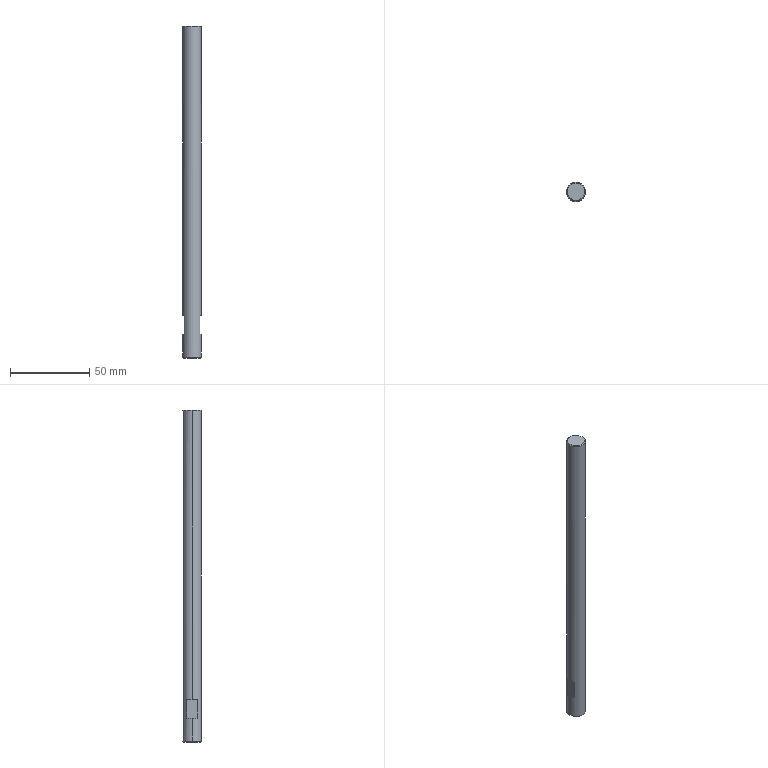Part | STEP file | 2010 Bag feed support shaft | 1 solid | 18 faces | box 12 x 12 x 210 mm | volume 23133 mm3 | plane 8 | cone 6 | cylinder 4 | commonest cylinder face diameters 5 x2 12 x2
STEP:
#1=CARTESIAN_POINT('',(0.,0.,0.));
#2=DIRECTION('',(0.,0.,1.));
#3=DIRECTION('',(1.,0.,0.));
#4=AXIS2_PLACEMENT_3D('',#1,#2,#3);
#5=CARTESIAN_POINT('',(5.5,0.,210.));
#6=VERTEX_POINT('',#5);
#7=CARTESIAN_POINT('',(-5.5,0.,210.));
#8=VERTEX_POINT('',#7);
#9=CARTESIAN_POINT('',(0.,0.,210.));
#10=DIRECTION('',(0.,0.,1.));
#11=DIRECTION('',(1.,0.,0.));
#12=AXIS2_PLACEMENT_3D('',#9,#10,#11);
#13=CIRCLE('',#12,5.5);
#14=CARTESIAN_POINT('',(0.,0.,210.));
#15=DIRECTION('',(0.,0.,-1.));
#16=DIRECTION('',(-1.,0.,0.));
#17=AXIS2_PLACEMENT_3D('',#14,#15,#16);
#18=CONICAL_SURFACE('',#17,5.5,0.7854);
#19=CARTESIAN_POINT('',(3.142,0.));
#20=DIRECTION('',(-1.,0.));
#21=VECTOR('',#20,1.);
#22=LINE('',#19,#21);
#23=(GEOMETRIC_REPRESENTATION_CONTEXT(2)PARAMETRIC_REPRESENTATION_CONTEXT()REPRESENTATION_CONTEXT('',''));
#24=DEFINITIONAL_REPRESENTATION('',(#22),#23);
#25=PCURVE('',#18,#24);
#26=CARTESIAN_POINT('',(0.,0.,210.));
#27=DIRECTION('',(0.,0.,1.));
#28=DIRECTION('',(1.,0.,0.));
#29=AXIS2_PLACEMENT_3D('',#26,#27,#28);
#30=PLANE('',#29);
#31=CARTESIAN_POINT('',(0.,0.));
#32=DIRECTION('',(1.,0.));
#33=AXIS2_PLACEMENT_2D('',#31,#32);
#34=CIRCLE('',#33,5.5);
#35=(GEOMETRIC_REPRESENTATION_CONTEXT(2)PARAMETRIC_REPRESENTATION_CONTEXT()REPRESENTATION_CONTEXT('',''));
#36=DEFINITIONAL_REPRESENTATION('',(#34),#35);
#37=PCURVE('',#30,#36);
#38=SURFACE_CURVE('',#13,(#25,#37),.PCURVE_S1.);
#39=EDGE_CURVE('',#6,#8,#38,.T.);
#40=ORIENTED_EDGE('',*,*,#39,.F.);
#41=CARTESIAN_POINT('',(6.,0.,209.5));
#42=VERTEX_POINT('',#41);
#43=CARTESIAN_POINT('',(5.5,0.,210.));
#44=DIRECTION('',(0.7071,0.,-0.7071));
#45=VECTOR('',#44,1.);
#46=LINE('',#43,#45);
#47=CARTESIAN_POINT('',(3.142,0.));
#48=DIRECTION('',(0.,1.));
#49=VECTOR('',#48,1.);
#50=LINE('',#47,#49);
#51=(GEOMETRIC_REPRESENTATION_CONTEXT(2)PARAMETRIC_REPRESENTATION_CONTEXT()REPRESENTATION_CONTEXT('',''));
#52=DEFINITIONAL_REPRESENTATION('',(#50),#51);
#53=PCURVE('',#18,#52);
#54=CARTESIAN_POINT('',(0.,0.,210.));
#55=DIRECTION('',(0.,0.,-1.));
#56=DIRECTION('',(-1.,0.,0.));
#57=AXIS2_PLACEMENT_3D('',#54,#55,#56);
#58=CONICAL_SURFACE('',#57,5.5,0.7854);
#59=CARTESIAN_POINT('',(3.142,0.));
#60=DIRECTION('',(0.,1.));
#61=VECTOR('',#60,1.);
#62=LINE('',#59,#61);
#63=(GEOMETRIC_REPRESENTATION_CONTEXT(2)PARAMETRIC_REPRESENTATION_CONTEXT()REPRESENTATION_CONTEXT('',''));
#64=DEFINITIONAL_REPRESENTATION('',(#62),#63);
#65=PCURVE('',#58,#64);
#66=SURFACE_CURVE('',#46,(#53,#65),.PCURVE_S1.);
#67=EDGE_CURVE('',#6,#42,#66,.T.);
#68=ORIENTED_EDGE('',*,*,#67,.T.);
#69=CARTESIAN_POINT('',(-6.,0.,209.5));
#70=VERTEX_POINT('',#69);
#71=CARTESIAN_POINT('',(0.,0.,209.5));
#72=DIRECTION('',(0.,0.,-1.));
#73=DIRECTION('',(1.,0.,0.));
#74=AXIS2_PLACEMENT_3D('',#71,#72,#73);
#75=CIRCLE('',#74,6.);
#76=CARTESIAN_POINT('',(-3.142,0.5));
#77=DIRECTION('',(1.,0.));
#78=VECTOR('',#77,1.);
#79=LINE('',#76,#78);
#80=(GEOMETRIC_REPRESENTATION_CONTEXT(2)PARAMETRIC_REPRESENTATION_CONTEXT()REPRESENTATION_CONTEXT('',''));
#81=DEFINITIONAL_REPRESENTATION('',(#79),#80);
#82=PCURVE('',#18,#81);
#83=CARTESIAN_POINT('',(0.,0.,210.));
#84=DIRECTION('',(0.,0.,-1.));
#85=DIRECTION('',(-1.,0.,0.));
#86=AXIS2_PLACEMENT_3D('',#83,#84,#85);
#87=CYLINDRICAL_SURFACE('',#86,6.);
#88=CARTESIAN_POINT('',(-3.142,0.5));
#89=DIRECTION('',(1.,0.));
#90=VECTOR('',#89,1.);
#91=LINE('',#88,#90);
#92=(GEOMETRIC_REPRESENTATION_CONTEXT(2)PARAMETRIC_REPRESENTATION_CONTEXT()REPRESENTATION_CONTEXT('',''));
#93=DEFINITIONAL_REPRESENTATION('',(#91),#92);
#94=PCURVE('',#87,#93);
#95=SURFACE_CURVE('',#75,(#82,#94),.PCURVE_S1.);
#96=EDGE_CURVE('',#70,#42,#95,.T.);
#97=ORIENTED_EDGE('',*,*,#96,.F.);
#98=CARTESIAN_POINT('',(-5.5,0.,210.));
#99=DIRECTION('',(-0.7071,0.,-0.7071));
#100=VECTOR('',#99,1.);
#101=LINE('',#98,#100);
#102=CARTESIAN_POINT('',(0.,0.));
#103=DIRECTION('',(0.,1.));
#104=VECTOR('',#103,1.);
#105=LINE('',#102,#104);
#106=(GEOMETRIC_REPRESENTATION_CONTEXT(2)PARAMETRIC_REPRESENTATION_CONTEXT()REPRESENTATION_CONTEXT('',''));
#107=DEFINITIONAL_REPRESENTATION('',(#105),#106);
#108=PCURVE('',#18,#107);
#109=CARTESIAN_POINT('',(6.283,0.));
#110=DIRECTION('',(0.,1.));
#111=VECTOR('',#110,1.);
#112=LINE('',#109,#111);
#113=(GEOMETRIC_REPRESENTATION_CONTEXT(2)PARAMETRIC_REPRESENTATION_CONTEXT()REPRESENTATION_CONTEXT('',''));
#114=DEFINITIONAL_REPRESENTATION('',(#112),#113);
#115=PCURVE('',#58,#114);
#116=SURFACE_CURVE('',#101,(#108,#115),.PCURVE_S1.);
#117=EDGE_CURVE('',#8,#70,#116,.T.);
#118=ORIENTED_EDGE('',*,*,#117,.F.);
#119=EDGE_LOOP('',(#40,#68,#97,#118));
#120=FACE_BOUND('',#119,.T.);
#121=ADVANCED_FACE('',(#120),#18,.T.);
#122=CARTESIAN_POINT('',(-5.5,0.,0.));
#123=VERTEX_POINT('',#122);
#124=CARTESIAN_POINT('',(5.5,0.,0.));
#125=VERTEX_POINT('',#124);
#126=CARTESIAN_POINT('',(0.,0.,0.));
#127=DIRECTION('',(0.,0.,-1.));
#128=DIRECTION('',(1.,0.,0.));
#129=AXIS2_PLACEMENT_3D('',#126,#127,#128);
#130=CIRCLE('',#129,5.5);
#131=CARTESIAN_POINT('',(0.,0.,0.5));
#132=DIRECTION('',(0.,0.,1.));
#133=DIRECTION('',(1.,0.,0.));
#134=AXIS2_PLACEMENT_3D('',#131,#132,#133);
#135=CONICAL_SURFACE('',#134,6.,0.7854);
#136=CARTESIAN_POINT('',(6.283,-0.5));
#137=DIRECTION('',(-1.,0.));
#138=VECTOR('',#137,1.);
#139=LINE('',#136,#138);
#140=(GEOMETRIC_REPRESENTATION_CONTEXT(2)PARAMETRIC_REPRESENTATION_CONTEXT()REPRESENTATION_CONTEXT('',''));
#141=DEFINITIONAL_REPRESENTATION('',(#139),#140);
#142=PCURVE('',#135,#141);
#143=CARTESIAN_POINT('',(0.,0.,0.));
#144=DIRECTION('',(0.,0.,1.));
#145=DIRECTION('',(1.,0.,0.));
#146=AXIS2_PLACEMENT_3D('',#143,#144,#145);
#147=PLANE('',#146);
#148=CARTESIAN_POINT('',(5.5,0.));
#149=CARTESIAN_POINT('',(5.5,-9.526));
#150=CARTESIAN_POINT('',(-2.75,-4.763));
#151=CARTESIAN_POINT('',(-11.,0.));
#152=CARTESIAN_POINT('',(-2.75,4.763));
#153=CARTESIAN_POINT('',(5.5,9.526));
#154=CARTESIAN_POINT('',(5.5,0.));
#155=(BOUNDED_CURVE()B_SPLINE_CURVE(2,(#148,#149,#150,#151,#152,#153,#154),.UNSPECIFIED.,.T.,.F.)B_SPLINE_CURVE_WITH_KNOTS((1,2,2,2,2,1),(-2.094,0.,2.094,4.189,6.283,8.378),.UNSPECIFIED.)CURVE()GEOMETRIC_REPRESENTATION_ITEM()RATIONAL_B_SPLINE_CURVE((1.,0.5,1.,0.5,1.,0.5,1.))REPRESENTATION_ITEM(''));
#156=(GEOMETRIC_REPRESENTATION_CONTEXT(2)PARAMETRIC_REPRESENTATION_CONTEXT()REPRESENTATION_CONTEXT('',''));
#157=DEFINITIONAL_REPRESENTATION('',(#155),#156);
#158=PCURVE('',#147,#157);
#159=SURFACE_CURVE('',#130,(#142,#158),.PCURVE_S1.);
#160=EDGE_CURVE('',#123,#125,#159,.T.);
#161=ORIENTED_EDGE('',*,*,#160,.F.);
#162=CARTESIAN_POINT('',(-6.,0.,0.5));
#163=VERTEX_POINT('',#162);
#164=CARTESIAN_POINT('',(-6.,0.,0.5));
#165=DIRECTION('',(-0.7071,0.,0.7071));
#166=VECTOR('',#165,1.);
#167=LINE('',#164,#166);
#168=CARTESIAN_POINT('',(3.142,0.));
#169=DIRECTION('',(0.,1.));
#170=VECTOR('',#169,1.);
#171=LINE('',#168,#170);
#172=(GEOMETRIC_REPRESENTATION_CONTEXT(2)PARAMETRIC_REPRESENTATION_CONTEXT()REPRESENTATION_CONTEXT('',''));
#173=DEFINITIONAL_REPRESENTATION('',(#171),#172);
#174=PCURVE('',#135,#173);
#175=CARTESIAN_POINT('',(0.,0.,0.5));
#176=DIRECTION('',(0.,0.,1.));
#177=DIRECTION('',(1.,0.,0.));
#178=AXIS2_PLACEMENT_3D('',#175,#176,#177);
#179=CONICAL_SURFACE('',#178,6.,0.7854);
#180=CARTESIAN_POINT('',(3.142,0.));
#181=DIRECTION('',(0.,1.));
#182=VECTOR('',#181,1.);
#183=LINE('',#180,#182);
#184=(GEOMETRIC_REPRESENTATION_CONTEXT(2)PARAMETRIC_REPRESENTATION_CONTEXT()REPRESENTATION_CONTEXT('',''));
#185=DEFINITIONAL_REPRESENTATION('',(#183),#184);
#186=PCURVE('',#179,#185);
#187=SURFACE_CURVE('',#167,(#174,#186),.PCURVE_S1.);
#188=EDGE_CURVE('',#123,#163,#187,.T.);
#189=ORIENTED_EDGE('',*,*,#188,.T.);
#190=CARTESIAN_POINT('',(6.,0.,0.5));
#191=VERTEX_POINT('',#190);
#192=CARTESIAN_POINT('',(0.,0.,0.5));
#193=DIRECTION('',(0.,0.,1.));
#194=DIRECTION('',(1.,0.,0.));
#195=AXIS2_PLACEMENT_3D('',#192,#193,#194);
#196=CIRCLE('',#195,6.);
#197=CARTESIAN_POINT('',(0.,0.));
#198=DIRECTION('',(1.,0.));
#199=VECTOR('',#198,1.);
#200=LINE('',#197,#199);
#201=(GEOMETRIC_REPRESENTATION_CONTEXT(2)PARAMETRIC_REPRESENTATION_CONTEXT()REPRESENTATION_CONTEXT('',''));
#202=DEFINITIONAL_REPRESENTATION('',(#200),#201);
#203=PCURVE('',#135,#202);
#204=CARTESIAN_POINT('',(3.142,209.5));
#205=DIRECTION('',(-1.,0.));
#206=VECTOR('',#205,1.);
#207=LINE('',#204,#206);
#208=(GEOMETRIC_REPRESENTATION_CONTEXT(2)PARAMETRIC_REPRESENTATION_CONTEXT()REPRESENTATION_CONTEXT('',''));
#209=DEFINITIONAL_REPRESENTATION('',(#207),#208);
#210=PCURVE('',#87,#209);
#211=SURFACE_CURVE('',#196,(#203,#210),.PCURVE_S1.);
#212=EDGE_CURVE('',#191,#163,#211,.T.);
#213=ORIENTED_EDGE('',*,*,#212,.F.);
#214=CARTESIAN_POINT('',(6.,0.,0.5));
#215=DIRECTION('',(0.7071,0.,0.7071));
#216=VECTOR('',#215,1.);
#217=LINE('',#214,#216);
#218=CARTESIAN_POINT('',(0.,0.));
#219=DIRECTION('',(0.,1.));
#220=VECTOR('',#219,1.);
#221=LINE('',#218,#220);
#222=(GEOMETRIC_REPRESENTATION_CONTEXT(2)PARAMETRIC_REPRESENTATION_CONTEXT()REPRESENTATION_CONTEXT('',''));
#223=DEFINITIONAL_REPRESENTATION('',(#221),#222);
#224=PCURVE('',#135,#223);
#225=CARTESIAN_POINT('',(6.283,0.));
#226=DIRECTION('',(0.,1.));
#227=VECTOR('',#226,1.);
#228=LINE('',#225,#227);
#229=(GEOMETRIC_REPRESENTATION_CONTEXT(2)PARAMETRIC_REPRESENTATION_CONTEXT()REPRESENTATION_CONTEXT('',''));
#230=DEFINITIONAL_REPRESENTATION('',(#228),#229);
#231=PCURVE('',#179,#230);
#232=SURFACE_CURVE('',#217,(#224,#231),.PCURVE_S1.);
#233=EDGE_CURVE('',#125,#191,#232,.T.);
#234=ORIENTED_EDGE('',*,*,#233,.F.);
#235=EDGE_LOOP('',(#161,#189,#213,#234));
#236=FACE_BOUND('',#235,.T.);
#237=ADVANCED_FACE('',(#236),#135,.T.);
#238=CARTESIAN_POINT('',(-2.5,0.,25.));
#239=VERTEX_POINT('',#238);
#240=CARTESIAN_POINT('',(-2.5,0.,0.));
#241=VERTEX_POINT('',#240);
#242=CARTESIAN_POINT('',(-2.5,0.,0.));
#243=DIRECTION('',(0.,0.,-1.));
#244=VECTOR('',#243,1.);
#245=LINE('',#242,#244);
#246=CARTESIAN_POINT('',(0.,0.,0.));
#247=DIRECTION('',(0.,0.,-1.));
#248=DIRECTION('',(-1.,0.,0.));
#249=AXIS2_PLACEMENT_3D('',#246,#247,#248);
#250=CYLINDRICAL_SURFACE('',#249,2.5);
#251=CARTESIAN_POINT('',(6.283,0.));
#252=DIRECTION('',(0.,1.));
#253=VECTOR('',#252,1.);
#254=LINE('',#251,#253);
#255=(GEOMETRIC_REPRESENTATION_CONTEXT(2)PARAMETRIC_REPRESENTATION_CONTEXT()REPRESENTATION_CONTEXT('',''));
#256=DEFINITIONAL_REPRESENTATION('',(#254),#255);
#257=PCURVE('',#250,#256);
#258=CARTESIAN_POINT('',(0.,0.,0.));
#259=DIRECTION('',(0.,0.,-1.));
#260=DIRECTION('',(-1.,0.,0.));
#261=AXIS2_PLACEMENT_3D('',#258,#259,#260);
#262=CYLINDRICAL_SURFACE('',#261,2.5);
#263=CARTESIAN_POINT('',(0.,0.));
#264=DIRECTION('',(0.,1.));
#265=VECTOR('',#264,1.);
#266=LINE('',#263,#265);
#267=(GEOMETRIC_REPRESENTATION_CONTEXT(2)PARAMETRIC_REPRESENTATION_CONTEXT()REPRESENTATION_CONTEXT('',''));
#268=DEFINITIONAL_REPRESENTATION('',(#266),#267);
#269=PCURVE('',#262,#268);
#270=SURFACE_CURVE('',#245,(#257,#269),.PCURVE_S1.);
#271=EDGE_CURVE('',#239,#241,#270,.T.);
#272=ORIENTED_EDGE('',*,*,#271,.T.);
#273=CARTESIAN_POINT('',(2.5,0.,0.));
#274=VERTEX_POINT('',#273);
#275=CARTESIAN_POINT('',(0.,0.,0.));
#276=DIRECTION('',(0.,0.,-1.));
#277=DIRECTION('',(-1.,0.,0.));
#278=AXIS2_PLACEMENT_3D('',#275,#276,#277);
#279=CIRCLE('',#278,2.5);
#280=CARTESIAN_POINT('',(0.,0.));
#281=DIRECTION('',(1.,0.));
#282=VECTOR('',#281,1.);
#283=LINE('',#280,#282);
#284=(GEOMETRIC_REPRESENTATION_CONTEXT(2)PARAMETRIC_REPRESENTATION_CONTEXT()REPRESENTATION_CONTEXT('',''));
#285=DEFINITIONAL_REPRESENTATION('',(#283),#284);
#286=PCURVE('',#250,#285);
#287=CARTESIAN_POINT('',(-2.5,0.));
#288=CARTESIAN_POINT('',(-2.5,4.33));
#289=CARTESIAN_POINT('',(1.25,2.165));
#290=CARTESIAN_POINT('',(5.,0.));
#291=CARTESIAN_POINT('',(1.25,-2.165));
#292=CARTESIAN_POINT('',(-2.5,-4.33));
#293=CARTESIAN_POINT('',(-2.5,0.));
#294=(BOUNDED_CURVE()B_SPLINE_CURVE(2,(#287,#288,#289,#290,#291,#292,#293),.UNSPECIFIED.,.T.,.F.)B_SPLINE_CURVE_WITH_KNOTS((1,2,2,2,2,1),(-2.094,0.,2.094,4.189,6.283,8.378),.UNSPECIFIED.)CURVE()GEOMETRIC_REPRESENTATION_ITEM()RATIONAL_B_SPLINE_CURVE((1.,0.5,1.,0.5,1.,0.5,1.))REPRESENTATION_ITEM(''));
#295=(GEOMETRIC_REPRESENTATION_CONTEXT(2)PARAMETRIC_REPRESENTATION_CONTEXT()REPRESENTATION_CONTEXT('',''));
#296=DEFINITIONAL_REPRESENTATION('',(#294),#295);
#297=PCURVE('',#147,#296);
#298=SURFACE_CURVE('',#279,(#286,#297),.PCURVE_S1.);
#299=EDGE_CURVE('',#274,#241,#298,.T.);
#300=ORIENTED_EDGE('',*,*,#299,.F.);
#301=CARTESIAN_POINT('',(2.5,0.,25.));
#302=VERTEX_POINT('',#301);
#303=CARTESIAN_POINT('',(2.5,0.,0.));
#304=DIRECTION('',(0.,0.,-1.));
#305=VECTOR('',#304,1.);
#306=LINE('',#303,#305);
#307=CARTESIAN_POINT('',(3.142,0.));
#308=DIRECTION('',(0.,1.));
#309=VECTOR('',#308,1.);
#310=LINE('',#307,#309);
#311=(GEOMETRIC_REPRESENTATION_CONTEXT(2)PARAMETRIC_REPRESENTATION_CONTEXT()REPRESENTATION_CONTEXT('',''));
#312=DEFINITIONAL_REPRESENTATION('',(#310),#311);
#313=PCURVE('',#250,#312);
#314=CARTESIAN_POINT('',(3.142,0.));
#315=DIRECTION('',(0.,1.));
#316=VECTOR('',#315,1.);
#317=LINE('',#314,#316);
#318=(GEOMETRIC_REPRESENTATION_CONTEXT(2)PARAMETRIC_REPRESENTATION_CONTEXT()REPRESENTATION_CONTEXT('',''));
#319=DEFINITIONAL_REPRESENTATION('',(#317),#318);
#320=PCURVE('',#262,#319);
#321=SURFACE_CURVE('',#306,(#313,#320),.PCURVE_S1.);
#322=EDGE_CURVE('',#302,#274,#321,.T.);
#323=ORIENTED_EDGE('',*,*,#322,.F.);
#324=CARTESIAN_POINT('',(0.,0.,25.));
#325=DIRECTION('',(0.,0.,-1.));
#326=DIRECTION('',(-1.,0.,0.));
#327=AXIS2_PLACEMENT_3D('',#324,#325,#326);
#328=CIRCLE('',#327,2.5);
#329=CARTESIAN_POINT('',(0.,-25.));
#330=DIRECTION('',(1.,0.));
#331=VECTOR('',#330,1.);
#332=LINE('',#329,#331);
#333=(GEOMETRIC_REPRESENTATION_CONTEXT(2)PARAMETRIC_REPRESENTATION_CONTEXT()REPRESENTATION_CONTEXT('',''));
#334=DEFINITIONAL_REPRESENTATION('',(#332),#333);
#335=PCURVE('',#250,#334);
#336=CARTESIAN_POINT('',(0.,0.,25.));
#337=DIRECTION('',(0.,0.,-1.));
#338=DIRECTION('',(-1.,0.,0.));
#339=AXIS2_PLACEMENT_3D('',#336,#337,#338);
#340=CONICAL_SURFACE('',#339,2.5,1.03);
#341=CARTESIAN_POINT('',(0.,0.));
#342=DIRECTION('',(1.,0.));
#343=VECTOR('',#342,1.);
#344=LINE('',#341,#343);
#345=(GEOMETRIC_REPRESENTATION_CONTEXT(2)PARAMETRIC_REPRESENTATION_CONTEXT()REPRESENTATION_CONTEXT('',''));
#346=DEFINITIONAL_REPRESENTATION('',(#344),#345);
#347=PCURVE('',#340,#346);
#348=SURFACE_CURVE('',#328,(#335,#347),.PCURVE_S1.);
#349=EDGE_CURVE('',#302,#239,#348,.T.);
#350=ORIENTED_EDGE('',*,*,#349,.T.);
#351=EDGE_LOOP('',(#272,#300,#323,#350));
#352=FACE_BOUND('',#351,.F.);
#353=ADVANCED_FACE('',(#352),#250,.F.);
#354=ORIENTED_EDGE('',*,*,#349,.F.);
#355=CARTESIAN_POINT('',(0.,0.,26.502));
#356=VERTEX_POINT('',#355);
#357=CARTESIAN_POINT('',(2.5,0.,25.));
#358=DIRECTION('',(0.8572,0.,-0.515));
#359=VECTOR('',#358,1.);
#360=LINE('',#357,#359);
#361=CARTESIAN_POINT('',(3.142,0.));
#362=DIRECTION('',(0.,1.));
#363=VECTOR('',#362,1.);
#364=LINE('',#361,#363);
#365=(GEOMETRIC_REPRESENTATION_CONTEXT(2)PARAMETRIC_REPRESENTATION_CONTEXT()REPRESENTATION_CONTEXT('',''));
#366=DEFINITIONAL_REPRESENTATION('',(#364),#365);
#367=PCURVE('',#340,#366);
#368=CARTESIAN_POINT('',(0.,0.,25.));
#369=DIRECTION('',(0.,0.,-1.));
#370=DIRECTION('',(-1.,0.,0.));
#371=AXIS2_PLACEMENT_3D('',#368,#369,#370);
#372=CONICAL_SURFACE('',#371,2.5,1.03);
#373=CARTESIAN_POINT('',(3.142,0.));
#374=DIRECTION('',(0.,1.));
#375=VECTOR('',#374,1.);
#376=LINE('',#373,#375);
#377=(GEOMETRIC_REPRESENTATION_CONTEXT(2)PARAMETRIC_REPRESENTATION_CONTEXT()REPRESENTATION_CONTEXT('',''));
#378=DEFINITIONAL_REPRESENTATION('',(#376),#377);
#379=PCURVE('',#372,#378);
#380=SURFACE_CURVE('',#360,(#367,#379),.PCURVE_S1.);
#381=EDGE_CURVE('',#356,#302,#380,.T.);
#382=ORIENTED_EDGE('',*,*,#381,.F.);
#383=CARTESIAN_POINT('',(-2.5,0.,25.));
#384=DIRECTION('',(-0.8572,0.,-0.515));
#385=VECTOR('',#384,1.);
#386=LINE('',#383,#385);
#387=CARTESIAN_POINT('',(6.283,0.));
#388=DIRECTION('',(0.,1.));
#389=VECTOR('',#388,1.);
#390=LINE('',#387,#389);
#391=(GEOMETRIC_REPRESENTATION_CONTEXT(2)PARAMETRIC_REPRESENTATION_CONTEXT()REPRESENTATION_CONTEXT('',''));
#392=DEFINITIONAL_REPRESENTATION('',(#390),#391);
#393=PCURVE('',#340,#392);
#394=CARTESIAN_POINT('',(0.,0.));
#395=DIRECTION('',(0.,1.));
#396=VECTOR('',#395,1.);
#397=LINE('',#394,#396);
#398=(GEOMETRIC_REPRESENTATION_CONTEXT(2)PARAMETRIC_REPRESENTATION_CONTEXT()REPRESENTATION_CONTEXT('',''));
#399=DEFINITIONAL_REPRESENTATION('',(#397),#398);
#400=PCURVE('',#372,#399);
#401=SURFACE_CURVE('',#386,(#393,#400),.PCURVE_S1.);
#402=EDGE_CURVE('',#356,#239,#401,.T.);
#403=ORIENTED_EDGE('',*,*,#402,.T.);
#404=EDGE_LOOP('',(#354,#382,#403));
#405=FACE_BOUND('',#404,.F.);
#406=ADVANCED_FACE('',(#405),#340,.F.);
#407=ORIENTED_EDGE('',*,*,#96,.T.);
#408=CARTESIAN_POINT('',(6.,0.,27.));
#409=VERTEX_POINT('',#408);
#410=CARTESIAN_POINT('',(6.,0.,210.));
#411=DIRECTION('',(0.,0.,-1.));
#412=VECTOR('',#411,1.);
#413=LINE('',#410,#412);
#414=CARTESIAN_POINT('',(3.142,0.));
#415=DIRECTION('',(0.,1.));
#416=VECTOR('',#415,1.);
#417=LINE('',#414,#416);
#418=(GEOMETRIC_REPRESENTATION_CONTEXT(2)PARAMETRIC_REPRESENTATION_CONTEXT()REPRESENTATION_CONTEXT('',''));
#419=DEFINITIONAL_REPRESENTATION('',(#417),#418);
#420=PCURVE('',#87,#419);
#421=CARTESIAN_POINT('',(0.,0.,210.));
#422=DIRECTION('',(0.,0.,-1.));
#423=DIRECTION('',(-1.,0.,0.));
#424=AXIS2_PLACEMENT_3D('',#421,#422,#423);
#425=CYLINDRICAL_SURFACE('',#424,6.);
#426=CARTESIAN_POINT('',(3.142,0.));
#427=DIRECTION('',(0.,1.));
#428=VECTOR('',#427,1.);
#429=LINE('',#426,#428);
#430=(GEOMETRIC_REPRESENTATION_CONTEXT(2)PARAMETRIC_REPRESENTATION_CONTEXT()REPRESENTATION_CONTEXT('',''));
#431=DEFINITIONAL_REPRESENTATION('',(#429),#430);
#432=PCURVE('',#425,#431);
#433=SURFACE_CURVE('',#413,(#420,#432),.PCURVE_S1.);
#434=EDGE_CURVE('',#42,#409,#433,.T.);
#435=ORIENTED_EDGE('',*,*,#434,.T.);
#436=CARTESIAN_POINT('',(5.,3.317,27.));
#437=VERTEX_POINT('',#436);
#438=CARTESIAN_POINT('',(0.,0.,27.));
#439=DIRECTION('',(0.,0.,-1.));
#440=DIRECTION('',(-1.,0.,0.));
#441=AXIS2_PLACEMENT_3D('',#438,#439,#440);
#442=CIRCLE('',#441,6.);
#443=CARTESIAN_POINT('',(0.,183.));
#444=DIRECTION('',(1.,0.));
#445=VECTOR('',#444,1.);
#446=LINE('',#443,#445);
#447=(GEOMETRIC_REPRESENTATION_CONTEXT(2)PARAMETRIC_REPRESENTATION_CONTEXT()REPRESENTATION_CONTEXT('',''));
#448=DEFINITIONAL_REPRESENTATION('',(#446),#447);
#449=PCURVE('',#87,#448);
#450=CARTESIAN_POINT('',(5.,10.,27.));
#451=DIRECTION('',(0.,0.,-1.));
#452=DIRECTION('',(-1.,0.,0.));
#453=AXIS2_PLACEMENT_3D('',#450,#451,#452);
#454=PLANE('',#453);
#455=CARTESIAN_POINT('',(5.,-10.));
#456=DIRECTION('',(1.,0.));
#457=AXIS2_PLACEMENT_2D('',#455,#456);
#458=CIRCLE('',#457,6.);
#459=(GEOMETRIC_REPRESENTATION_CONTEXT(2)PARAMETRIC_REPRESENTATION_CONTEXT()REPRESENTATION_CONTEXT('',''));
#460=DEFINITIONAL_REPRESENTATION('',(#458),#459);
#461=PCURVE('',#454,#460);
#462=SURFACE_CURVE('',#442,(#449,#461),.PCURVE_S1.);
#463=EDGE_CURVE('',#437,#409,#462,.T.);
#464=ORIENTED_EDGE('',*,*,#463,.F.);
#465=CARTESIAN_POINT('',(5.,3.317,15.));
#466=VERTEX_POINT('',#465);
#467=CARTESIAN_POINT('',(5.,3.317,210.));
#468=DIRECTION('',(0.,0.,1.));
#469=VECTOR('',#468,1.);
#470=LINE('',#467,#469);
#471=CARTESIAN_POINT('',(2.556,0.));
#472=DIRECTION('',(0.,-1.));
#473=VECTOR('',#472,1.);
#474=LINE('',#471,#473);
#475=(GEOMETRIC_REPRESENTATION_CONTEXT(2)PARAMETRIC_REPRESENTATION_CONTEXT()REPRESENTATION_CONTEXT('',''));
#476=DEFINITIONAL_REPRESENTATION('',(#474),#475);
#477=PCURVE('',#87,#476);
#478=CARTESIAN_POINT('',(5.,10.,27.));
#479=DIRECTION('',(1.,0.,0.));
#480=DIRECTION('',(0.,0.,-1.));
#481=AXIS2_PLACEMENT_3D('',#478,#479,#480);
#482=PLANE('',#481);
#483=CARTESIAN_POINT('',(-183.,-6.683));
#484=DIRECTION('',(-1.,0.));
#485=VECTOR('',#484,1.);
#486=LINE('',#483,#485);
#487=(GEOMETRIC_REPRESENTATION_CONTEXT(2)PARAMETRIC_REPRESENTATION_CONTEXT()REPRESENTATION_CONTEXT('',''));
#488=DEFINITIONAL_REPRESENTATION('',(#486),#487);
#489=PCURVE('',#482,#488);
#490=SURFACE_CURVE('',#470,(#477,#489),.PCURVE_S1.);
#491=EDGE_CURVE('',#466,#437,#490,.T.);
#492=ORIENTED_EDGE('',*,*,#491,.F.);
#493=CARTESIAN_POINT('',(6.,0.,15.));
#494=VERTEX_POINT('',#493);
#495=CARTESIAN_POINT('',(0.,0.,15.));
#496=DIRECTION('',(0.,0.,1.));
#497=DIRECTION('',(1.,0.,0.));
#498=AXIS2_PLACEMENT_3D('',#495,#496,#497);
#499=CIRCLE('',#498,6.);
#500=CARTESIAN_POINT('',(3.142,195.));
#501=DIRECTION('',(-1.,0.));
#502=VECTOR('',#501,1.);
#503=LINE('',#500,#502);
#504=(GEOMETRIC_REPRESENTATION_CONTEXT(2)PARAMETRIC_REPRESENTATION_CONTEXT()REPRESENTATION_CONTEXT('',''));
#505=DEFINITIONAL_REPRESENTATION('',(#503),#504);
#506=PCURVE('',#87,#505);
#507=CARTESIAN_POINT('',(5.,10.,15.));
#508=DIRECTION('',(0.,0.,1.));
#509=DIRECTION('',(1.,0.,0.));
#510=AXIS2_PLACEMENT_3D('',#507,#508,#509);
#511=PLANE('',#510);
#512=CARTESIAN_POINT('',(-5.,-10.));
#513=DIRECTION('',(1.,0.));
#514=AXIS2_PLACEMENT_2D('',#512,#513);
#515=CIRCLE('',#514,6.);
#516=(GEOMETRIC_REPRESENTATION_CONTEXT(2)PARAMETRIC_REPRESENTATION_CONTEXT()REPRESENTATION_CONTEXT('',''));
#517=DEFINITIONAL_REPRESENTATION('',(#515),#516);
#518=PCURVE('',#511,#517);
#519=SURFACE_CURVE('',#499,(#506,#518),.PCURVE_S1.);
#520=EDGE_CURVE('',#494,#466,#519,.T.);
#521=ORIENTED_EDGE('',*,*,#520,.F.);
#522=CARTESIAN_POINT('',(6.,0.,210.));
#523=DIRECTION('',(0.,0.,-1.));
#524=VECTOR('',#523,1.);
#525=LINE('',#522,#524);
#526=CARTESIAN_POINT('',(3.142,0.));
#527=DIRECTION('',(0.,1.));
#528=VECTOR('',#527,1.);
#529=LINE('',#526,#528);
#530=(GEOMETRIC_REPRESENTATION_CONTEXT(2)PARAMETRIC_REPRESENTATION_CONTEXT()REPRESENTATION_CONTEXT('',''));
#531=DEFINITIONAL_REPRESENTATION('',(#529),#530);
#532=PCURVE('',#87,#531);
#533=CARTESIAN_POINT('',(3.142,0.));
#534=DIRECTION('',(0.,1.));
#535=VECTOR('',#534,1.);
#536=LINE('',#533,#535);
#537=(GEOMETRIC_REPRESENTATION_CONTEXT(2)PARAMETRIC_REPRESENTATION_CONTEXT()REPRESENTATION_CONTEXT('',''));
#538=DEFINITIONAL_REPRESENTATION('',(#536),#537);
#539=PCURVE('',#425,#538);
#540=SURFACE_CURVE('',#525,(#532,#539),.PCURVE_S1.);
#541=EDGE_CURVE('',#494,#191,#540,.T.);
#542=ORIENTED_EDGE('',*,*,#541,.T.);
#543=ORIENTED_EDGE('',*,*,#212,.T.);
#544=CARTESIAN_POINT('',(-6.,0.,15.));
#545=VERTEX_POINT('',#544);
#546=CARTESIAN_POINT('',(-6.,0.,210.));
#547=DIRECTION('',(0.,0.,-1.));
#548=VECTOR('',#547,1.);
#549=LINE('',#546,#548);
#550=CARTESIAN_POINT('',(0.,0.));
#551=DIRECTION('',(0.,1.));
#552=VECTOR('',#551,1.);
#553=LINE('',#550,#552);
#554=(GEOMETRIC_REPRESENTATION_CONTEXT(2)PARAMETRIC_REPRESENTATION_CONTEXT()REPRESENTATION_CONTEXT('',''));
#555=DEFINITIONAL_REPRESENTATION('',(#553),#554);
#556=PCURVE('',#87,#555);
#557=CARTESIAN_POINT('',(6.283,0.));
#558=DIRECTION('',(0.,1.));
#559=VECTOR('',#558,1.);
#560=LINE('',#557,#559);
#561=(GEOMETRIC_REPRESENTATION_CONTEXT(2)PARAMETRIC_REPRESENTATION_CONTEXT()REPRESENTATION_CONTEXT('',''));
#562=DEFINITIONAL_REPRESENTATION('',(#560),#561);
#563=PCURVE('',#425,#562);
#564=SURFACE_CURVE('',#549,(#556,#563),.PCURVE_S1.);
#565=EDGE_CURVE('',#545,#163,#564,.T.);
#566=ORIENTED_EDGE('',*,*,#565,.F.);
#567=CARTESIAN_POINT('',(-5.,3.317,15.));
#568=VERTEX_POINT('',#567);
#569=CARTESIAN_POINT('',(0.,0.,15.));
#570=DIRECTION('',(0.,0.,1.));
#571=DIRECTION('',(1.,0.,0.));
#572=AXIS2_PLACEMENT_3D('',#569,#570,#571);
#573=CIRCLE('',#572,6.);
#574=CARTESIAN_POINT('',(3.142,195.));
#575=DIRECTION('',(-1.,0.));
#576=VECTOR('',#575,1.);
#577=LINE('',#574,#576);
#578=(GEOMETRIC_REPRESENTATION_CONTEXT(2)PARAMETRIC_REPRESENTATION_CONTEXT()REPRESENTATION_CONTEXT('',''));
#579=DEFINITIONAL_REPRESENTATION('',(#577),#578);
#580=PCURVE('',#87,#579);
#581=CARTESIAN_POINT('',(-14.949,10.,15.));
#582=DIRECTION('',(0.,0.,1.));
#583=DIRECTION('',(1.,0.,0.));
#584=AXIS2_PLACEMENT_3D('',#581,#582,#583);
#585=PLANE('',#584);
#586=CARTESIAN_POINT('',(14.949,-10.));
#587=DIRECTION('',(1.,0.));
#588=AXIS2_PLACEMENT_2D('',#586,#587);
#589=CIRCLE('',#588,6.);
#590=(GEOMETRIC_REPRESENTATION_CONTEXT(2)PARAMETRIC_REPRESENTATION_CONTEXT()REPRESENTATION_CONTEXT('',''));
#591=DEFINITIONAL_REPRESENTATION('',(#589),#590);
#592=PCURVE('',#585,#591);
#593=SURFACE_CURVE('',#573,(#580,#592),.PCURVE_S1.);
#594=EDGE_CURVE('',#568,#545,#593,.T.);
#595=ORIENTED_EDGE('',*,*,#594,.F.);
#596=CARTESIAN_POINT('',(-5.,3.317,27.));
#597=VERTEX_POINT('',#596);
#598=CARTESIAN_POINT('',(-5.,3.317,210.));
#599=DIRECTION('',(0.,0.,-1.));
#600=VECTOR('',#599,1.);
#601=LINE('',#598,#600);
#602=CARTESIAN_POINT('',(0.5857,0.));
#603=DIRECTION('',(0.,1.));
#604=VECTOR('',#603,1.);
#605=LINE('',#602,#604);
#606=(GEOMETRIC_REPRESENTATION_CONTEXT(2)PARAMETRIC_REPRESENTATION_CONTEXT()REPRESENTATION_CONTEXT('',''));
#607=DEFINITIONAL_REPRESENTATION('',(#605),#606);
#608=PCURVE('',#87,#607);
#609=CARTESIAN_POINT('',(-5.,10.,27.));
#610=DIRECTION('',(-1.,0.,0.));
#611=DIRECTION('',(0.,0.,1.));
#612=AXIS2_PLACEMENT_3D('',#609,#610,#611);
#613=PLANE('',#612);
#614=CARTESIAN_POINT('',(183.,-6.683));
#615=DIRECTION('',(-1.,0.));
#616=VECTOR('',#615,1.);
#617=LINE('',#614,#616);
#618=(GEOMETRIC_REPRESENTATION_CONTEXT(2)PARAMETRIC_REPRESENTATION_CONTEXT()REPRESENTATION_CONTEXT('',''));
#619=DEFINITIONAL_REPRESENTATION('',(#617),#618);
#620=PCURVE('',#613,#619);
#621=SURFACE_CURVE('',#601,(#608,#620),.PCURVE_S1.);
#622=EDGE_CURVE('',#597,#568,#621,.T.);
#623=ORIENTED_EDGE('',*,*,#622,.F.);
#624=CARTESIAN_POINT('',(-6.,0.,27.));
#625=VERTEX_POINT('',#624);
#626=CARTESIAN_POINT('',(0.,0.,27.));
#627=DIRECTION('',(0.,0.,-1.));
#628=DIRECTION('',(-1.,0.,0.));
#629=AXIS2_PLACEMENT_3D('',#626,#627,#628);
#630=CIRCLE('',#629,6.);
#631=CARTESIAN_POINT('',(0.,183.));
#632=DIRECTION('',(1.,0.));
#633=VECTOR('',#632,1.);
#634=LINE('',#631,#633);
#635=(GEOMETRIC_REPRESENTATION_CONTEXT(2)PARAMETRIC_REPRESENTATION_CONTEXT()REPRESENTATION_CONTEXT('',''));
#636=DEFINITIONAL_REPRESENTATION('',(#634),#635);
#637=PCURVE('',#87,#636);
#638=CARTESIAN_POINT('',(-14.949,10.,27.));
#639=DIRECTION('',(0.,0.,-1.));
#640=DIRECTION('',(-1.,0.,0.));
#641=AXIS2_PLACEMENT_3D('',#638,#639,#640);
#642=PLANE('',#641);
#643=CARTESIAN_POINT('',(-14.949,-10.));
#644=DIRECTION('',(1.,0.));
#645=AXIS2_PLACEMENT_2D('',#643,#644);
#646=CIRCLE('',#645,6.);
#647=(GEOMETRIC_REPRESENTATION_CONTEXT(2)PARAMETRIC_REPRESENTATION_CONTEXT()REPRESENTATION_CONTEXT('',''));
#648=DEFINITIONAL_REPRESENTATION('',(#646),#647);
#649=PCURVE('',#642,#648);
#650=SURFACE_CURVE('',#630,(#637,#649),.PCURVE_S1.);
#651=EDGE_CURVE('',#625,#597,#650,.T.);
#652=ORIENTED_EDGE('',*,*,#651,.F.);
#653=CARTESIAN_POINT('',(-6.,0.,210.));
#654=DIRECTION('',(0.,0.,-1.));
#655=VECTOR('',#654,1.);
#656=LINE('',#653,#655);
#657=CARTESIAN_POINT('',(0.,0.));
#658=DIRECTION('',(0.,1.));
#659=VECTOR('',#658,1.);
#660=LINE('',#657,#659);
#661=(GEOMETRIC_REPRESENTATION_CONTEXT(2)PARAMETRIC_REPRESENTATION_CONTEXT()REPRESENTATION_CONTEXT('',''));
#662=DEFINITIONAL_REPRESENTATION('',(#660),#661);
#663=PCURVE('',#87,#662);
#664=CARTESIAN_POINT('',(6.283,0.));
#665=DIRECTION('',(0.,1.));
#666=VECTOR('',#665,1.);
#667=LINE('',#664,#666);
#668=(GEOMETRIC_REPRESENTATION_CONTEXT(2)PARAMETRIC_REPRESENTATION_CONTEXT()REPRESENTATION_CONTEXT('',''));
#669=DEFINITIONAL_REPRESENTATION('',(#667),#668);
#670=PCURVE('',#425,#669);
#671=SURFACE_CURVE('',#656,(#663,#670),.PCURVE_S1.);
#672=EDGE_CURVE('',#70,#625,#671,.T.);
#673=ORIENTED_EDGE('',*,*,#672,.F.);
#674=EDGE_LOOP('',(#407,#435,#464,#492,#521,#542,#543,#566,#595,#623,#652,#673));
#675=FACE_BOUND('',#674,.T.);
#676=ADVANCED_FACE('',(#675),#87,.T.);
#677=ORIENTED_EDGE('',*,*,#434,.F.);
#678=CARTESIAN_POINT('',(0.,0.,209.5));
#679=DIRECTION('',(0.,0.,-1.));
#680=DIRECTION('',(1.,0.,0.));
#681=AXIS2_PLACEMENT_3D('',#678,#679,#680);
#682=CIRCLE('',#681,6.);
#683=CARTESIAN_POINT('',(3.142,0.5));
#684=DIRECTION('',(1.,0.));
#685=VECTOR('',#684,1.);
#686=LINE('',#683,#685);
#687=(GEOMETRIC_REPRESENTATION_CONTEXT(2)PARAMETRIC_REPRESENTATION_CONTEXT()REPRESENTATION_CONTEXT('',''));
#688=DEFINITIONAL_REPRESENTATION('',(#686),#687);
#689=PCURVE('',#425,#688);
#690=CARTESIAN_POINT('',(3.142,0.5));
#691=DIRECTION('',(1.,0.));
#692=VECTOR('',#691,1.);
#693=LINE('',#690,#692);
#694=(GEOMETRIC_REPRESENTATION_CONTEXT(2)PARAMETRIC_REPRESENTATION_CONTEXT()REPRESENTATION_CONTEXT('',''));
#695=DEFINITIONAL_REPRESENTATION('',(#693),#694);
#696=PCURVE('',#58,#695);
#697=SURFACE_CURVE('',#682,(#689,#696),.PCURVE_S1.);
#698=EDGE_CURVE('',#42,#70,#697,.T.);
#699=ORIENTED_EDGE('',*,*,#698,.T.);
#700=ORIENTED_EDGE('',*,*,#672,.T.);
#701=CARTESIAN_POINT('',(-5.,-3.317,27.));
#702=VERTEX_POINT('',#701);
#703=CARTESIAN_POINT('',(0.,0.,27.));
#704=DIRECTION('',(0.,0.,-1.));
#705=DIRECTION('',(-1.,0.,0.));
#706=AXIS2_PLACEMENT_3D('',#703,#704,#705);
#707=CIRCLE('',#706,6.);
#708=CARTESIAN_POINT('',(0.,183.));
#709=DIRECTION('',(1.,0.));
#710=VECTOR('',#709,1.);
#711=LINE('',#708,#710);
#712=(GEOMETRIC_REPRESENTATION_CONTEXT(2)PARAMETRIC_REPRESENTATION_CONTEXT()REPRESENTATION_CONTEXT('',''));
#713=DEFINITIONAL_REPRESENTATION('',(#711),#712);
#714=PCURVE('',#425,#713);
#715=CARTESIAN_POINT('',(-14.949,-10.));
#716=DIRECTION('',(1.,0.));
#717=AXIS2_PLACEMENT_2D('',#715,#716);
#718=CIRCLE('',#717,6.);
#719=(GEOMETRIC_REPRESENTATION_CONTEXT(2)PARAMETRIC_REPRESENTATION_CONTEXT()REPRESENTATION_CONTEXT('',''));
#720=DEFINITIONAL_REPRESENTATION('',(#718),#719);
#721=PCURVE('',#642,#720);
#722=SURFACE_CURVE('',#707,(#714,#721),.PCURVE_S1.);
#723=EDGE_CURVE('',#702,#625,#722,.T.);
#724=ORIENTED_EDGE('',*,*,#723,.F.);
#725=CARTESIAN_POINT('',(-5.,-3.317,15.));
#726=VERTEX_POINT('',#725);
#727=CARTESIAN_POINT('',(-5.,-3.317,210.));
#728=DIRECTION('',(0.,0.,1.));
#729=VECTOR('',#728,1.);
#730=LINE('',#727,#729);
#731=CARTESIAN_POINT('',(5.697,0.));
#732=DIRECTION('',(0.,-1.));
#733=VECTOR('',#732,1.);
#734=LINE('',#731,#733);
#735=(GEOMETRIC_REPRESENTATION_CONTEXT(2)PARAMETRIC_REPRESENTATION_CONTEXT()REPRESENTATION_CONTEXT('',''));
#736=DEFINITIONAL_REPRESENTATION('',(#734),#735);
#737=PCURVE('',#425,#736);
#738=CARTESIAN_POINT('',(183.,-13.317));
#739=DIRECTION('',(1.,0.));
#740=VECTOR('',#739,1.);
#741=LINE('',#738,#740);
#742=(GEOMETRIC_REPRESENTATION_CONTEXT(2)PARAMETRIC_REPRESENTATION_CONTEXT()REPRESENTATION_CONTEXT('',''));
#743=DEFINITIONAL_REPRESENTATION('',(#741),#742);
#744=PCURVE('',#613,#743);
#745=SURFACE_CURVE('',#730,(#737,#744),.PCURVE_S1.);
#746=EDGE_CURVE('',#726,#702,#745,.T.);
#747=ORIENTED_EDGE('',*,*,#746,.F.);
#748=CARTESIAN_POINT('',(0.,0.,15.));
#749=DIRECTION('',(0.,0.,1.));
#750=DIRECTION('',(1.,0.,0.));
#751=AXIS2_PLACEMENT_3D('',#748,#749,#750);
#752=CIRCLE('',#751,6.);
#753=CARTESIAN_POINT('',(9.425,195.));
#754=DIRECTION('',(-1.,0.));
#755=VECTOR('',#754,1.);
#756=LINE('',#753,#755);
#757=(GEOMETRIC_REPRESENTATION_CONTEXT(2)PARAMETRIC_REPRESENTATION_CONTEXT()REPRESENTATION_CONTEXT('',''));
#758=DEFINITIONAL_REPRESENTATION('',(#756),#757);
#759=PCURVE('',#425,#758);
#760=CARTESIAN_POINT('',(14.949,-10.));
#761=DIRECTION('',(1.,0.));
#762=AXIS2_PLACEMENT_2D('',#760,#761);
#763=CIRCLE('',#762,6.);
#764=(GEOMETRIC_REPRESENTATION_CONTEXT(2)PARAMETRIC_REPRESENTATION_CONTEXT()REPRESENTATION_CONTEXT('',''));
#765=DEFINITIONAL_REPRESENTATION('',(#763),#764);
#766=PCURVE('',#585,#765);
#767=SURFACE_CURVE('',#752,(#759,#766),.PCURVE_S1.);
#768=EDGE_CURVE('',#545,#726,#767,.T.);
#769=ORIENTED_EDGE('',*,*,#768,.F.);
#770=ORIENTED_EDGE('',*,*,#565,.T.);
#771=CARTESIAN_POINT('',(0.,0.,0.5));
#772=DIRECTION('',(0.,0.,1.));
#773=DIRECTION('',(1.,0.,0.));
#774=AXIS2_PLACEMENT_3D('',#771,#772,#773);
#775=CIRCLE('',#774,6.);
#776=CARTESIAN_POINT('',(9.425,209.5));
#777=DIRECTION('',(-1.,0.));
#778=VECTOR('',#777,1.);
#779=LINE('',#776,#778);
#780=(GEOMETRIC_REPRESENTATION_CONTEXT(2)PARAMETRIC_REPRESENTATION_CONTEXT()REPRESENTATION_CONTEXT('',''));
#781=DEFINITIONAL_REPRESENTATION('',(#779),#780);
#782=PCURVE('',#425,#781);
#783=CARTESIAN_POINT('',(0.,0.));
#784=DIRECTION('',(1.,0.));
#785=VECTOR('',#784,1.);
#786=LINE('',#783,#785);
#787=(GEOMETRIC_REPRESENTATION_CONTEXT(2)PARAMETRIC_REPRESENTATION_CONTEXT()REPRESENTATION_CONTEXT('',''));
#788=DEFINITIONAL_REPRESENTATION('',(#786),#787);
#789=PCURVE('',#179,#788);
#790=SURFACE_CURVE('',#775,(#782,#789),.PCURVE_S1.);
#791=EDGE_CURVE('',#163,#191,#790,.T.);
#792=ORIENTED_EDGE('',*,*,#791,.T.);
#793=ORIENTED_EDGE('',*,*,#541,.F.);
#794=CARTESIAN_POINT('',(5.,-3.317,15.));
#795=VERTEX_POINT('',#794);
#796=CARTESIAN_POINT('',(0.,0.,15.));
#797=DIRECTION('',(0.,0.,1.));
#798=DIRECTION('',(1.,0.,0.));
#799=AXIS2_PLACEMENT_3D('',#796,#797,#798);
#800=CIRCLE('',#799,6.);
#801=CARTESIAN_POINT('',(9.425,195.));
#802=DIRECTION('',(-1.,0.));
#803=VECTOR('',#802,1.);
#804=LINE('',#801,#803);
#805=(GEOMETRIC_REPRESENTATION_CONTEXT(2)PARAMETRIC_REPRESENTATION_CONTEXT()REPRESENTATION_CONTEXT('',''));
#806=DEFINITIONAL_REPRESENTATION('',(#804),#805);
#807=PCURVE('',#425,#806);
#808=CARTESIAN_POINT('',(-5.,-10.));
#809=DIRECTION('',(1.,0.));
#810=AXIS2_PLACEMENT_2D('',#808,#809);
#811=CIRCLE('',#810,6.);
#812=(GEOMETRIC_REPRESENTATION_CONTEXT(2)PARAMETRIC_REPRESENTATION_CONTEXT()REPRESENTATION_CONTEXT('',''));
#813=DEFINITIONAL_REPRESENTATION('',(#811),#812);
#814=PCURVE('',#511,#813);
#815=SURFACE_CURVE('',#800,(#807,#814),.PCURVE_S1.);
#816=EDGE_CURVE('',#795,#494,#815,.T.);
#817=ORIENTED_EDGE('',*,*,#816,.F.);
#818=CARTESIAN_POINT('',(5.,-3.317,27.));
#819=VERTEX_POINT('',#818);
#820=CARTESIAN_POINT('',(5.,-3.317,210.));
#821=DIRECTION('',(0.,0.,-1.));
#822=VECTOR('',#821,1.);
#823=LINE('',#820,#822);
#824=CARTESIAN_POINT('',(3.727,0.));
#825=DIRECTION('',(0.,1.));
#826=VECTOR('',#825,1.);
#827=LINE('',#824,#826);
#828=(GEOMETRIC_REPRESENTATION_CONTEXT(2)PARAMETRIC_REPRESENTATION_CONTEXT()REPRESENTATION_CONTEXT('',''));
#829=DEFINITIONAL_REPRESENTATION('',(#827),#828);
#830=PCURVE('',#425,#829);
#831=CARTESIAN_POINT('',(-183.,-13.317));
#832=DIRECTION('',(1.,0.));
#833=VECTOR('',#832,1.);
#834=LINE('',#831,#833);
#835=(GEOMETRIC_REPRESENTATION_CONTEXT(2)PARAMETRIC_REPRESENTATION_CONTEXT()REPRESENTATION_CONTEXT('',''));
#836=DEFINITIONAL_REPRESENTATION('',(#834),#835);
#837=PCURVE('',#482,#836);
#838=SURFACE_CURVE('',#823,(#830,#837),.PCURVE_S1.);
#839=EDGE_CURVE('',#819,#795,#838,.T.);
#840=ORIENTED_EDGE('',*,*,#839,.F.);
#841=CARTESIAN_POINT('',(0.,0.,27.));
#842=DIRECTION('',(0.,0.,-1.));
#843=DIRECTION('',(-1.,0.,0.));
#844=AXIS2_PLACEMENT_3D('',#841,#842,#843);
#845=CIRCLE('',#844,6.);
#846=CARTESIAN_POINT('',(0.,183.));
#847=DIRECTION('',(1.,0.));
#848=VECTOR('',#847,1.);
#849=LINE('',#846,#848);
#850=(GEOMETRIC_REPRESENTATION_CONTEXT(2)PARAMETRIC_REPRESENTATION_CONTEXT()REPRESENTATION_CONTEXT('',''));
#851=DEFINITIONAL_REPRESENTATION('',(#849),#850);
#852=PCURVE('',#425,#851);
#853=CARTESIAN_POINT('',(5.,-10.));
#854=DIRECTION('',(1.,0.));
#855=AXIS2_PLACEMENT_2D('',#853,#854);
#856=CIRCLE('',#855,6.);
#857=(GEOMETRIC_REPRESENTATION_CONTEXT(2)PARAMETRIC_REPRESENTATION_CONTEXT()REPRESENTATION_CONTEXT('',''));
#858=DEFINITIONAL_REPRESENTATION('',(#856),#857);
#859=PCURVE('',#454,#858);
#860=SURFACE_CURVE('',#845,(#852,#859),.PCURVE_S1.);
#861=EDGE_CURVE('',#409,#819,#860,.T.);
#862=ORIENTED_EDGE('',*,*,#861,.F.);
#863=EDGE_LOOP('',(#677,#699,#700,#724,#747,#769,#770,#792,#793,#817,#840,#862));
#864=FACE_BOUND('',#863,.T.);
#865=ADVANCED_FACE('',(#864),#425,.T.);
#866=CARTESIAN_POINT('',(0.,0.,210.));
#867=DIRECTION('',(0.,0.,1.));
#868=DIRECTION('',(1.,0.,0.));
#869=AXIS2_PLACEMENT_3D('',#866,#867,#868);
#870=CIRCLE('',#869,5.5);
#871=CARTESIAN_POINT('',(0.,0.));
#872=DIRECTION('',(1.,0.));
#873=AXIS2_PLACEMENT_2D('',#871,#872);
#874=CIRCLE('',#873,5.5);
#875=(GEOMETRIC_REPRESENTATION_CONTEXT(2)PARAMETRIC_REPRESENTATION_CONTEXT()REPRESENTATION_CONTEXT('',''));
#876=DEFINITIONAL_REPRESENTATION('',(#874),#875);
#877=PCURVE('',#30,#876);
#878=CARTESIAN_POINT('',(9.425,0.));
#879=DIRECTION('',(-1.,0.));
#880=VECTOR('',#879,1.);
#881=LINE('',#878,#880);
#882=(GEOMETRIC_REPRESENTATION_CONTEXT(2)PARAMETRIC_REPRESENTATION_CONTEXT()REPRESENTATION_CONTEXT('',''));
#883=DEFINITIONAL_REPRESENTATION('',(#881),#882);
#884=PCURVE('',#58,#883);
#885=SURFACE_CURVE('',#870,(#877,#884),.PCURVE_S1.);
#886=EDGE_CURVE('',#8,#6,#885,.T.);
#887=ORIENTED_EDGE('',*,*,#886,.T.);
#888=ORIENTED_EDGE('',*,*,#39,.T.);
#889=EDGE_LOOP('',(#887,#888));
#890=FACE_BOUND('',#889,.T.);
#891=ADVANCED_FACE('',(#890),#30,.T.);
#892=CARTESIAN_POINT('',(0.,0.,0.));
#893=DIRECTION('',(0.,0.,-1.));
#894=DIRECTION('',(1.,0.,0.));
#895=AXIS2_PLACEMENT_3D('',#892,#893,#894);
#896=CIRCLE('',#895,5.5);
#897=CARTESIAN_POINT('',(5.5,0.));
#898=CARTESIAN_POINT('',(5.5,-9.526));
#899=CARTESIAN_POINT('',(-2.75,-4.763));
#900=CARTESIAN_POINT('',(-11.,0.));
#901=CARTESIAN_POINT('',(-2.75,4.763));
#902=CARTESIAN_POINT('',(5.5,9.526));
#903=CARTESIAN_POINT('',(5.5,0.));
#904=(BOUNDED_CURVE()B_SPLINE_CURVE(2,(#897,#898,#899,#900,#901,#902,#903),.UNSPECIFIED.,.T.,.F.)B_SPLINE_CURVE_WITH_KNOTS((1,2,2,2,2,1),(-2.094,0.,2.094,4.189,6.283,8.378),.UNSPECIFIED.)CURVE()GEOMETRIC_REPRESENTATION_ITEM()RATIONAL_B_SPLINE_CURVE((1.,0.5,1.,0.5,1.,0.5,1.))REPRESENTATION_ITEM(''));
#905=(GEOMETRIC_REPRESENTATION_CONTEXT(2)PARAMETRIC_REPRESENTATION_CONTEXT()REPRESENTATION_CONTEXT('',''));
#906=DEFINITIONAL_REPRESENTATION('',(#904),#905);
#907=PCURVE('',#147,#906);
#908=CARTESIAN_POINT('',(6.283,-0.5));
#909=DIRECTION('',(-1.,0.));
#910=VECTOR('',#909,1.);
#911=LINE('',#908,#910);
#912=(GEOMETRIC_REPRESENTATION_CONTEXT(2)PARAMETRIC_REPRESENTATION_CONTEXT()REPRESENTATION_CONTEXT('',''));
#913=DEFINITIONAL_REPRESENTATION('',(#911),#912);
#914=PCURVE('',#179,#913);
#915=SURFACE_CURVE('',#896,(#907,#914),.PCURVE_S1.);
#916=EDGE_CURVE('',#125,#123,#915,.T.);
#917=ORIENTED_EDGE('',*,*,#916,.T.);
#918=ORIENTED_EDGE('',*,*,#160,.T.);
#919=EDGE_LOOP('',(#917,#918));
#920=FACE_BOUND('',#919,.T.);
#921=CARTESIAN_POINT('',(0.,0.,0.));
#922=DIRECTION('',(0.,0.,-1.));
#923=DIRECTION('',(-1.,0.,0.));
#924=AXIS2_PLACEMENT_3D('',#921,#922,#923);
#925=CIRCLE('',#924,2.5);
#926=CARTESIAN_POINT('',(-2.5,0.));
#927=CARTESIAN_POINT('',(-2.5,4.33));
#928=CARTESIAN_POINT('',(1.25,2.165));
#929=CARTESIAN_POINT('',(5.,0.));
#930=CARTESIAN_POINT('',(1.25,-2.165));
#931=CARTESIAN_POINT('',(-2.5,-4.33));
#932=CARTESIAN_POINT('',(-2.5,0.));
#933=(BOUNDED_CURVE()B_SPLINE_CURVE(2,(#926,#927,#928,#929,#930,#931,#932),.UNSPECIFIED.,.T.,.F.)B_SPLINE_CURVE_WITH_KNOTS((1,2,2,2,2,1),(-2.094,0.,2.094,4.189,6.283,8.378),.UNSPECIFIED.)CURVE()GEOMETRIC_REPRESENTATION_ITEM()RATIONAL_B_SPLINE_CURVE((1.,0.5,1.,0.5,1.,0.5,1.))REPRESENTATION_ITEM(''));
#934=(GEOMETRIC_REPRESENTATION_CONTEXT(2)PARAMETRIC_REPRESENTATION_CONTEXT()REPRESENTATION_CONTEXT('',''));
#935=DEFINITIONAL_REPRESENTATION('',(#933),#934);
#936=PCURVE('',#147,#935);
#937=CARTESIAN_POINT('',(0.,0.));
#938=DIRECTION('',(1.,0.));
#939=VECTOR('',#938,1.);
#940=LINE('',#937,#939);
#941=(GEOMETRIC_REPRESENTATION_CONTEXT(2)PARAMETRIC_REPRESENTATION_CONTEXT()REPRESENTATION_CONTEXT('',''));
#942=DEFINITIONAL_REPRESENTATION('',(#940),#941);
#943=PCURVE('',#262,#942);
#944=SURFACE_CURVE('',#925,(#936,#943),.PCURVE_S1.);
#945=EDGE_CURVE('',#241,#274,#944,.T.);
#946=ORIENTED_EDGE('',*,*,#945,.F.);
#947=ORIENTED_EDGE('',*,*,#299,.F.);
#948=EDGE_LOOP('',(#946,#947));
#949=FACE_BOUND('',#948,.T.);
#950=ADVANCED_FACE('',(#920,#949),#147,.F.);
#951=CARTESIAN_POINT('',(0.,0.,25.));
#952=DIRECTION('',(0.,0.,-1.));
#953=DIRECTION('',(-1.,0.,0.));
#954=AXIS2_PLACEMENT_3D('',#951,#952,#953);
#955=CIRCLE('',#954,2.5);
#956=CARTESIAN_POINT('',(0.,0.));
#957=DIRECTION('',(1.,0.));
#958=VECTOR('',#957,1.);
#959=LINE('',#956,#958);
#960=(GEOMETRIC_REPRESENTATION_CONTEXT(2)PARAMETRIC_REPRESENTATION_CONTEXT()REPRESENTATION_CONTEXT('',''));
#961=DEFINITIONAL_REPRESENTATION('',(#959),#960);
#962=PCURVE('',#372,#961);
#963=CARTESIAN_POINT('',(0.,-25.));
#964=DIRECTION('',(1.,0.));
#965=VECTOR('',#964,1.);
#966=LINE('',#963,#965);
#967=(GEOMETRIC_REPRESENTATION_CONTEXT(2)PARAMETRIC_REPRESENTATION_CONTEXT()REPRESENTATION_CONTEXT('',''));
#968=DEFINITIONAL_REPRESENTATION('',(#966),#967);
#969=PCURVE('',#262,#968);
#970=SURFACE_CURVE('',#955,(#962,#969),.PCURVE_S1.);
#971=EDGE_CURVE('',#239,#302,#970,.T.);
#972=ORIENTED_EDGE('',*,*,#971,.F.);
#973=ORIENTED_EDGE('',*,*,#402,.F.);
#974=ORIENTED_EDGE('',*,*,#381,.T.);
#975=EDGE_LOOP('',(#972,#973,#974));
#976=FACE_BOUND('',#975,.F.);
#977=ADVANCED_FACE('',(#976),#372,.F.);
#978=ORIENTED_EDGE('',*,*,#945,.F.);
#979=ORIENTED_EDGE('',*,*,#271,.F.);
#980=ORIENTED_EDGE('',*,*,#971,.T.);
#981=ORIENTED_EDGE('',*,*,#322,.T.);
#982=EDGE_LOOP('',(#978,#979,#980,#981));
#983=FACE_BOUND('',#982,.F.);
#984=ADVANCED_FACE('',(#983),#262,.F.);
#985=ORIENTED_EDGE('',*,*,#188,.F.);
#986=ORIENTED_EDGE('',*,*,#916,.F.);
#987=ORIENTED_EDGE('',*,*,#233,.T.);
#988=ORIENTED_EDGE('',*,*,#791,.F.);
#989=EDGE_LOOP('',(#985,#986,#987,#988));
#990=FACE_BOUND('',#989,.T.);
#991=ADVANCED_FACE('',(#990),#179,.T.);
#992=ORIENTED_EDGE('',*,*,#67,.F.);
#993=ORIENTED_EDGE('',*,*,#886,.F.);
#994=ORIENTED_EDGE('',*,*,#117,.T.);
#995=ORIENTED_EDGE('',*,*,#698,.F.);
#996=EDGE_LOOP('',(#992,#993,#994,#995));
#997=FACE_BOUND('',#996,.T.);
#998=ADVANCED_FACE('',(#997),#58,.T.);
#999=ORIENTED_EDGE('',*,*,#723,.T.);
#1000=ORIENTED_EDGE('',*,*,#651,.T.);
#1001=CARTESIAN_POINT('',(-5.,10.,27.));
#1002=DIRECTION('',(0.,-1.,0.));
#1003=VECTOR('',#1002,1.);
#1004=LINE('',#1001,#1003);
#1005=CARTESIAN_POINT('',(-9.949,0.));
#1006=DIRECTION('',(0.,-1.));
#1007=VECTOR('',#1006,1.);
#1008=LINE('',#1005,#1007);
#1009=(GEOMETRIC_REPRESENTATION_CONTEXT(2)PARAMETRIC_REPRESENTATION_CONTEXT()REPRESENTATION_CONTEXT('',''));
#1010=DEFINITIONAL_REPRESENTATION('',(#1008),#1009);
#1011=PCURVE('',#642,#1010);
#1012=CARTESIAN_POINT('',(0.,0.));
#1013=DIRECTION('',(0.,-1.));
#1014=VECTOR('',#1013,1.);
#1015=LINE('',#1012,#1014);
#1016=(GEOMETRIC_REPRESENTATION_CONTEXT(2)PARAMETRIC_REPRESENTATION_CONTEXT()REPRESENTATION_CONTEXT('',''));
#1017=DEFINITIONAL_REPRESENTATION('',(#1015),#1016);
#1018=PCURVE('',#613,#1017);
#1019=SURFACE_CURVE('',#1004,(#1011,#1018),.PCURVE_S1.);
#1020=EDGE_CURVE('',#597,#702,#1019,.T.);
#1021=ORIENTED_EDGE('',*,*,#1020,.T.);
#1022=EDGE_LOOP('',(#999,#1000,#1021));
#1023=FACE_BOUND('',#1022,.T.);
#1024=ADVANCED_FACE('',(#1023),#642,.T.);
#1025=ORIENTED_EDGE('',*,*,#622,.T.);
#1026=CARTESIAN_POINT('',(-5.,10.,15.));
#1027=DIRECTION('',(0.,-1.,0.));
#1028=VECTOR('',#1027,1.);
#1029=LINE('',#1026,#1028);
#1030=CARTESIAN_POINT('',(-12.,0.));
#1031=DIRECTION('',(0.,-1.));
#1032=VECTOR('',#1031,1.);
#1033=LINE('',#1030,#1032);
#1034=(GEOMETRIC_REPRESENTATION_CONTEXT(2)PARAMETRIC_REPRESENTATION_CONTEXT()REPRESENTATION_CONTEXT('',''));
#1035=DEFINITIONAL_REPRESENTATION('',(#1033),#1034);
#1036=PCURVE('',#613,#1035);
#1037=CARTESIAN_POINT('',(9.949,0.));
#1038=DIRECTION('',(0.,-1.));
#1039=VECTOR('',#1038,1.);
#1040=LINE('',#1037,#1039);
#1041=(GEOMETRIC_REPRESENTATION_CONTEXT(2)PARAMETRIC_REPRESENTATION_CONTEXT()REPRESENTATION_CONTEXT('',''));
#1042=DEFINITIONAL_REPRESENTATION('',(#1040),#1041);
#1043=PCURVE('',#585,#1042);
#1044=SURFACE_CURVE('',#1029,(#1036,#1043),.PCURVE_S1.);
#1045=EDGE_CURVE('',#568,#726,#1044,.T.);
#1046=ORIENTED_EDGE('',*,*,#1045,.T.);
#1047=ORIENTED_EDGE('',*,*,#746,.T.);
#1048=ORIENTED_EDGE('',*,*,#1020,.F.);
#1049=EDGE_LOOP('',(#1025,#1046,#1047,#1048));
#1050=FACE_BOUND('',#1049,.T.);
#1051=ADVANCED_FACE('',(#1050),#613,.T.);
#1052=ORIENTED_EDGE('',*,*,#594,.T.);
#1053=ORIENTED_EDGE('',*,*,#768,.T.);
#1054=ORIENTED_EDGE('',*,*,#1045,.F.);
#1055=EDGE_LOOP('',(#1052,#1053,#1054));
#1056=FACE_BOUND('',#1055,.T.);
#1057=ADVANCED_FACE('',(#1056),#585,.T.);
#1058=ORIENTED_EDGE('',*,*,#839,.T.);
#1059=CARTESIAN_POINT('',(5.,10.,15.));
#1060=DIRECTION('',(0.,-1.,0.));
#1061=VECTOR('',#1060,1.);
#1062=LINE('',#1059,#1061);
#1063=CARTESIAN_POINT('',(12.,0.));
#1064=DIRECTION('',(0.,-1.));
#1065=VECTOR('',#1064,1.);
#1066=LINE('',#1063,#1065);
#1067=(GEOMETRIC_REPRESENTATION_CONTEXT(2)PARAMETRIC_REPRESENTATION_CONTEXT()REPRESENTATION_CONTEXT('',''));
#1068=DEFINITIONAL_REPRESENTATION('',(#1066),#1067);
#1069=PCURVE('',#482,#1068);
#1070=CARTESIAN_POINT('',(0.,0.));
#1071=DIRECTION('',(0.,-1.));
#1072=VECTOR('',#1071,1.);
#1073=LINE('',#1070,#1072);
#1074=(GEOMETRIC_REPRESENTATION_CONTEXT(2)PARAMETRIC_REPRESENTATION_CONTEXT()REPRESENTATION_CONTEXT('',''));
#1075=DEFINITIONAL_REPRESENTATION('',(#1073),#1074);
#1076=PCURVE('',#511,#1075);
#1077=SURFACE_CURVE('',#1062,(#1069,#1076),.PCURVE_S1.);
#1078=EDGE_CURVE('',#466,#795,#1077,.T.);
#1079=ORIENTED_EDGE('',*,*,#1078,.F.);
#1080=ORIENTED_EDGE('',*,*,#491,.T.);
#1081=CARTESIAN_POINT('',(5.,10.,27.));
#1082=DIRECTION('',(0.,-1.,0.));
#1083=VECTOR('',#1082,1.);
#1084=LINE('',#1081,#1083);
#1085=CARTESIAN_POINT('',(0.,0.));
#1086=DIRECTION('',(0.,-1.));
#1087=VECTOR('',#1086,1.);
#1088=LINE('',#1085,#1087);
#1089=(GEOMETRIC_REPRESENTATION_CONTEXT(2)PARAMETRIC_REPRESENTATION_CONTEXT()REPRESENTATION_CONTEXT('',''));
#1090=DEFINITIONAL_REPRESENTATION('',(#1088),#1089);
#1091=PCURVE('',#482,#1090);
#1092=CARTESIAN_POINT('',(0.,0.));
#1093=DIRECTION('',(0.,-1.));
#1094=VECTOR('',#1093,1.);
#1095=LINE('',#1092,#1094);
#1096=(GEOMETRIC_REPRESENTATION_CONTEXT(2)PARAMETRIC_REPRESENTATION_CONTEXT()REPRESENTATION_CONTEXT('',''));
#1097=DEFINITIONAL_REPRESENTATION('',(#1095),#1096);
#1098=PCURVE('',#454,#1097);
#1099=SURFACE_CURVE('',#1084,(#1091,#1098),.PCURVE_S1.);
#1100=EDGE_CURVE('',#437,#819,#1099,.T.);
#1101=ORIENTED_EDGE('',*,*,#1100,.T.);
#1102=EDGE_LOOP('',(#1058,#1079,#1080,#1101));
#1103=FACE_BOUND('',#1102,.T.);
#1104=ADVANCED_FACE('',(#1103),#482,.T.);
#1105=ORIENTED_EDGE('',*,*,#463,.T.);
#1106=ORIENTED_EDGE('',*,*,#861,.T.);
#1107=ORIENTED_EDGE('',*,*,#1100,.F.);
#1108=EDGE_LOOP('',(#1105,#1106,#1107));
#1109=FACE_BOUND('',#1108,.T.);
#1110=ADVANCED_FACE('',(#1109),#454,.T.);
#1111=ORIENTED_EDGE('',*,*,#816,.T.);
#1112=ORIENTED_EDGE('',*,*,#520,.T.);
#1113=ORIENTED_EDGE('',*,*,#1078,.T.);
#1114=EDGE_LOOP('',(#1111,#1112,#1113));
#1115=FACE_BOUND('',#1114,.T.);
#1116=ADVANCED_FACE('',(#1115),#511,.T.);
#1117=CLOSED_SHELL('',(#121,#237,#353,#406,#676,#865,#891,#950,#977,#984,#991,#998,#1024,#1051,#1057,#1104,#1110,#1116));
#1118=MANIFOLD_SOLID_BREP('',#1117);
#1119=(LENGTH_UNIT()NAMED_UNIT(*)SI_UNIT(.MILLI.,.METRE.));
#1120=UNCERTAINTY_MEASURE_WITH_UNIT(LENGTH_MEASURE(0.0000001),#1119,'','');
#1121=(NAMED_UNIT(*)PLANE_ANGLE_UNIT()SI_UNIT($,.RADIAN.));
#1122=(NAMED_UNIT(*)SI_UNIT($,.STERADIAN.)SOLID_ANGLE_UNIT());
#1123=(GEOMETRIC_REPRESENTATION_CONTEXT(3)GLOBAL_UNCERTAINTY_ASSIGNED_CONTEXT((#1120))GLOBAL_UNIT_ASSIGNED_CONTEXT((#1119,#1121,#1122))REPRESENTATION_CONTEXT('',''));
#1124=ADVANCED_BREP_SHAPE_REPRESENTATION('',(#4,#1118),#1123);